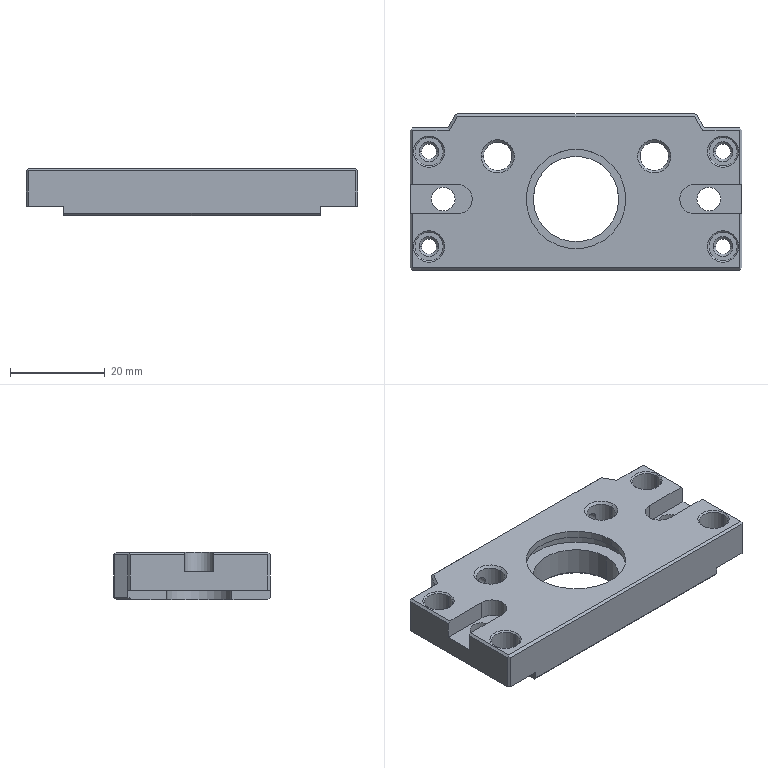Part | 1 solid | 126 faces | box 70 x 33 x 10 mm | volume 16070 mm3 | plane 50 | cylinder 42 | cone 34 | commonest cylinder face diameters 6 x12 2.4 x8 3.2 x8 5 x4 6.2 x2 14 x2